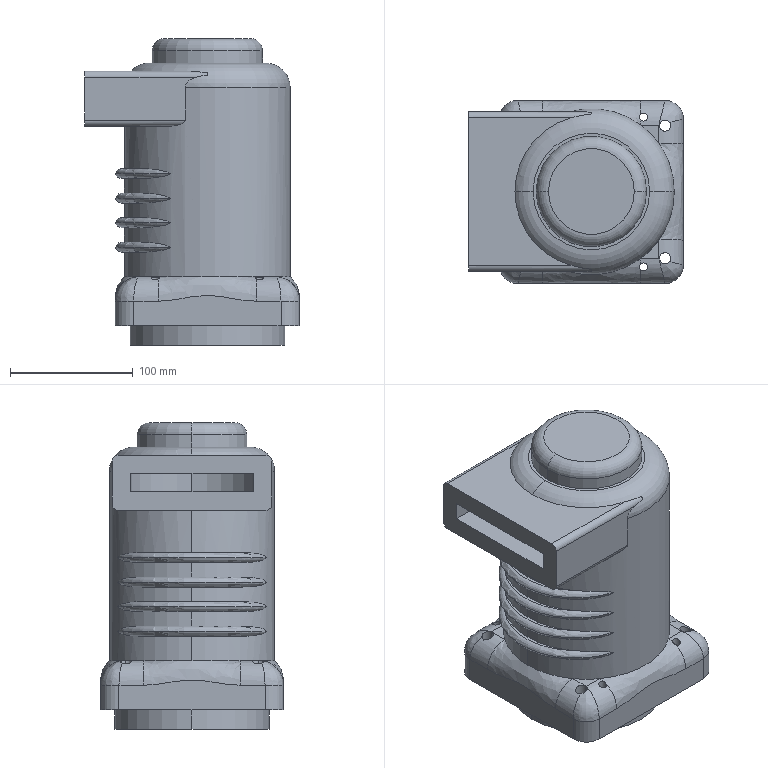Part | STEP file | Contact box type 150 | 1 solid | 92 faces | box 175.003 x 149 x 250 mm | volume 1890847 mm3 | cylinder 40 | plane 32 | torus 12 | spline 8 | commonest cylinder face diameters 6.5 x8 9.2 x8 40 x8 10 x4 30 x4 90 x2